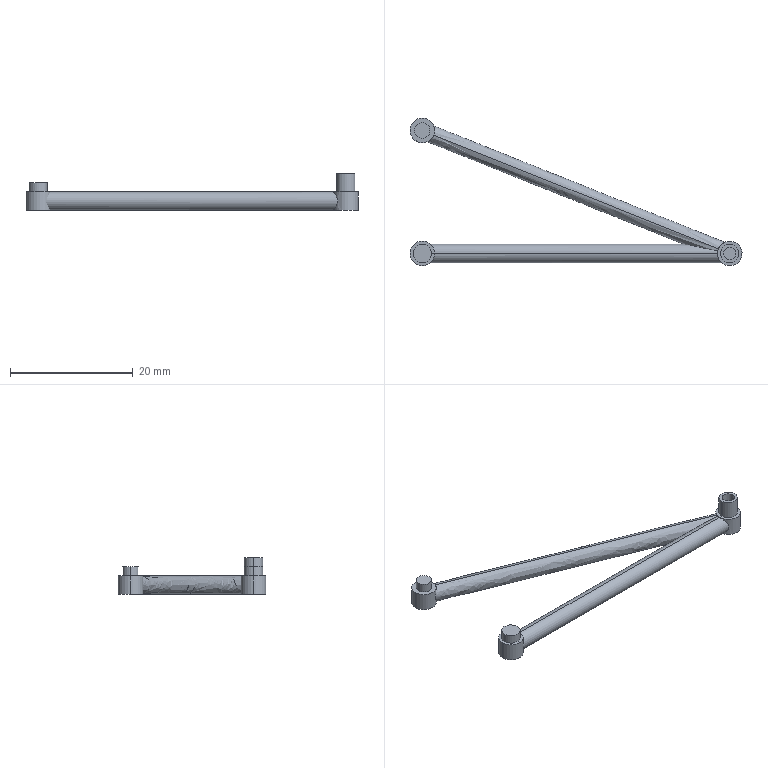Part | SolidWorks | features MirrorStock 1 | 3 solids | 36 faces | box 54 x 24 x 5.96 mm | volume 800.323 mm3 | cylinder 21 | plane 13 | spline 2 | commonest cylinder face diameters 4 x9 3 x6 0.5 x2 2 x2 2.5 x2
STEP:
#1=CARTESIAN_POINT('',(-2.,0.,-1.5));
#2=VERTEX_POINT('',#1);
#3=CARTESIAN_POINT('',(2.,0.,-1.5));
#4=VERTEX_POINT('',#3);
#5=CARTESIAN_POINT('',(0.,0.,-1.5));
#6=DIRECTION('',(0.,0.,1.));
#7=DIRECTION('',(1.,0.,0.));
#8=AXIS2_PLACEMENT_3D('',#5,#6,#7);
#9=CIRCLE('',#8,2.);
#10=EDGE_CURVE('',#2,#4,#9,.T.);
#11=ORIENTED_EDGE('',*,*,#10,.T.);
#12=CARTESIAN_POINT('',(2.,0.,1.5));
#13=VERTEX_POINT('',#12);
#14=CARTESIAN_POINT('',(2.,0.,-1.5));
#15=DIRECTION('',(0.,0.,1.));
#16=VECTOR('',#15,1000.);
#17=LINE('',#14,#16);
#18=EDGE_CURVE('',#4,#13,#17,.T.);
#19=ORIENTED_EDGE('',*,*,#18,.T.);
#20=CARTESIAN_POINT('',(-2.,0.,1.5));
#21=VERTEX_POINT('',#20);
#22=CARTESIAN_POINT('',(0.,0.,1.5));
#23=DIRECTION('',(0.,0.,1.));
#24=DIRECTION('',(1.,0.,0.));
#25=AXIS2_PLACEMENT_3D('',#22,#23,#24);
#26=CIRCLE('',#25,2.);
#27=EDGE_CURVE('',#21,#13,#26,.T.);
#28=ORIENTED_EDGE('',*,*,#27,.F.);
#29=CARTESIAN_POINT('',(-2.,0.,-1.5));
#30=DIRECTION('',(0.,0.,1.));
#31=VECTOR('',#30,1000.);
#32=LINE('',#29,#31);
#33=EDGE_CURVE('',#2,#21,#32,.T.);
#34=ORIENTED_EDGE('',*,*,#33,.F.);
#35=EDGE_LOOP('',(#11,#19,#28,#34));
#36=FACE_OUTER_BOUND('',#35,.T.);
#37=CARTESIAN_POINT('',(0.,0.,-1.5));
#38=DIRECTION('',(0.,0.,1.));
#39=DIRECTION('',(-1.,0.,0.));
#40=AXIS2_PLACEMENT_3D('',#37,#38,#39);
#41=CYLINDRICAL_SURFACE('',#40,2.);
#42=ADVANCED_FACE('',(#36),#41,.T.);
#43=ORIENTED_EDGE('',*,*,#18,.F.);
#44=CARTESIAN_POINT('',(0.,0.,-1.5));
#45=DIRECTION('',(0.,0.,1.));
#46=DIRECTION('',(1.,0.,0.));
#47=AXIS2_PLACEMENT_3D('',#44,#45,#46);
#48=CIRCLE('',#47,2.);
#49=EDGE_CURVE('',#4,#2,#48,.T.);
#50=ORIENTED_EDGE('',*,*,#49,.T.);
#51=ORIENTED_EDGE('',*,*,#33,.T.);
#52=CARTESIAN_POINT('',(0.,0.,1.5));
#53=DIRECTION('',(0.,0.,1.));
#54=DIRECTION('',(1.,0.,0.));
#55=AXIS2_PLACEMENT_3D('',#52,#53,#54);
#56=CIRCLE('',#55,2.);
#57=EDGE_CURVE('',#13,#21,#56,.T.);
#58=ORIENTED_EDGE('',*,*,#57,.F.);
#59=EDGE_LOOP('',(#43,#50,#51,#58));
#60=FACE_OUTER_BOUND('',#59,.T.);
#61=CARTESIAN_POINT('',(0.,0.,-1.5));
#62=DIRECTION('',(0.,0.,1.));
#63=DIRECTION('',(-1.,0.,0.));
#64=AXIS2_PLACEMENT_3D('',#61,#62,#63);
#65=CYLINDRICAL_SURFACE('',#64,2.);
#66=ADVANCED_FACE('',(#60),#65,.T.);
#67=ORIENTED_EDGE('',*,*,#10,.F.);
#68=ORIENTED_EDGE('',*,*,#49,.F.);
#69=EDGE_LOOP('',(#67,#68));
#70=FACE_OUTER_BOUND('',#69,.T.);
#71=CARTESIAN_POINT('',(0.,0.,-1.5));
#72=DIRECTION('',(0.,0.,-1.));
#73=DIRECTION('',(1.,0.,0.));
#74=AXIS2_PLACEMENT_3D('',#71,#72,#73);
#75=PLANE('',#74);
#76=ADVANCED_FACE('',(#70),#75,.T.);
#77=ORIENTED_EDGE('',*,*,#27,.T.);
#78=ORIENTED_EDGE('',*,*,#57,.T.);
#79=EDGE_LOOP('',(#77,#78));
#80=FACE_OUTER_BOUND('',#79,.T.);
#81=CARTESIAN_POINT('',(0.,0.,1.5));
#82=DIRECTION('',(0.,0.,-1.));
#83=DIRECTION('',(1.,0.,0.));
#84=AXIS2_PLACEMENT_3D('',#81,#82,#83);
#85=PLANE('',#84);
#86=ADVANCED_FACE('',(#80),#85,.F.);
#87=CLOSED_SHELL('',(#42,#66,#76,#86));
#88=MANIFOLD_SOLID_BREP('',#87);
#89=CARTESIAN_POINT('',(1.5,0.,3.));
#90=VERTEX_POINT('',#89);
#91=CARTESIAN_POINT('',(-1.5,0.,3.));
#92=VERTEX_POINT('',#91);
#93=CARTESIAN_POINT('',(0.,0.,3.));
#94=DIRECTION('',(0.,0.,-1.));
#95=DIRECTION('',(-1.,0.,0.));
#96=AXIS2_PLACEMENT_3D('',#93,#94,#95);
#97=CIRCLE('',#96,1.5);
#98=EDGE_CURVE('',#90,#92,#97,.T.);
#99=ORIENTED_EDGE('',*,*,#98,.T.);
#100=CARTESIAN_POINT('',(-1.5,0.,1.5));
#101=VERTEX_POINT('',#100);
#102=CARTESIAN_POINT('',(-1.5,0.,3.));
#103=DIRECTION('',(0.,0.,-1.));
#104=VECTOR('',#103,1000.);
#105=LINE('',#102,#104);
#106=EDGE_CURVE('',#92,#101,#105,.T.);
#107=ORIENTED_EDGE('',*,*,#106,.T.);
#108=CARTESIAN_POINT('',(1.5,0.,1.5));
#109=VERTEX_POINT('',#108);
#110=CARTESIAN_POINT('',(0.,0.,1.5));
#111=DIRECTION('',(0.,0.,-1.));
#112=DIRECTION('',(-1.,0.,0.));
#113=AXIS2_PLACEMENT_3D('',#110,#111,#112);
#114=CIRCLE('',#113,1.5);
#115=EDGE_CURVE('',#109,#101,#114,.T.);
#116=ORIENTED_EDGE('',*,*,#115,.F.);
#117=CARTESIAN_POINT('',(1.5,0.,3.));
#118=DIRECTION('',(0.,0.,-1.));
#119=VECTOR('',#118,1000.);
#120=LINE('',#117,#119);
#121=EDGE_CURVE('',#90,#109,#120,.T.);
#122=ORIENTED_EDGE('',*,*,#121,.F.);
#123=EDGE_LOOP('',(#99,#107,#116,#122));
#124=FACE_OUTER_BOUND('',#123,.T.);
#125=CARTESIAN_POINT('',(0.,0.,3.));
#126=DIRECTION('',(0.,0.,-1.));
#127=DIRECTION('',(1.,0.,0.));
#128=AXIS2_PLACEMENT_3D('',#125,#126,#127);
#129=CYLINDRICAL_SURFACE('',#128,1.5);
#130=ADVANCED_FACE('',(#124),#129,.T.);
#131=ORIENTED_EDGE('',*,*,#106,.F.);
#132=CARTESIAN_POINT('',(0.,0.,3.));
#133=DIRECTION('',(0.,0.,-1.));
#134=DIRECTION('',(-1.,0.,0.));
#135=AXIS2_PLACEMENT_3D('',#132,#133,#134);
#136=CIRCLE('',#135,1.5);
#137=EDGE_CURVE('',#92,#90,#136,.T.);
#138=ORIENTED_EDGE('',*,*,#137,.T.);
#139=ORIENTED_EDGE('',*,*,#121,.T.);
#140=CARTESIAN_POINT('',(0.,0.,1.5));
#141=DIRECTION('',(0.,0.,-1.));
#142=DIRECTION('',(-1.,0.,0.));
#143=AXIS2_PLACEMENT_3D('',#140,#141,#142);
#144=CIRCLE('',#143,1.5);
#145=EDGE_CURVE('',#101,#109,#144,.T.);
#146=ORIENTED_EDGE('',*,*,#145,.F.);
#147=EDGE_LOOP('',(#131,#138,#139,#146));
#148=FACE_OUTER_BOUND('',#147,.T.);
#149=CARTESIAN_POINT('',(0.,0.,3.));
#150=DIRECTION('',(0.,0.,-1.));
#151=DIRECTION('',(1.,0.,0.));
#152=AXIS2_PLACEMENT_3D('',#149,#150,#151);
#153=CYLINDRICAL_SURFACE('',#152,1.5);
#154=ADVANCED_FACE('',(#148),#153,.T.);
#155=ORIENTED_EDGE('',*,*,#98,.F.);
#156=ORIENTED_EDGE('',*,*,#137,.F.);
#157=EDGE_LOOP('',(#155,#156));
#158=FACE_OUTER_BOUND('',#157,.T.);
#159=CARTESIAN_POINT('',(0.,0.,3.));
#160=DIRECTION('',(0.,0.,1.));
#161=DIRECTION('',(-1.,0.,0.));
#162=AXIS2_PLACEMENT_3D('',#159,#160,#161);
#163=PLANE('',#162);
#164=ADVANCED_FACE('',(#158),#163,.T.);
#165=ORIENTED_EDGE('',*,*,#115,.T.);
#166=ORIENTED_EDGE('',*,*,#145,.T.);
#167=EDGE_LOOP('',(#165,#166));
#168=FACE_OUTER_BOUND('',#167,.T.);
#169=CARTESIAN_POINT('',(0.,0.,1.5));
#170=DIRECTION('',(0.,0.,1.));
#171=DIRECTION('',(-1.,0.,0.));
#172=AXIS2_PLACEMENT_3D('',#169,#170,#171);
#173=PLANE('',#172);
#174=ADVANCED_FACE('',(#168),#173,.F.);
#175=CLOSED_SHELL('',(#130,#154,#164,#174));
#176=MANIFOLD_SOLID_BREP('',#175);
#177=CARTESIAN_POINT('',(49.,0.,4.46));
#178=VERTEX_POINT('',#177);
#179=CARTESIAN_POINT('',(51.,0.,4.46));
#180=VERTEX_POINT('',#179);
#181=CARTESIAN_POINT('',(50.,0.,4.46));
#182=DIRECTION('',(0.,0.,-1.));
#183=DIRECTION('',(-1.,0.,0.));
#184=AXIS2_PLACEMENT_3D('',#181,#182,#183);
#185=CIRCLE('',#184,1.);
#186=EDGE_CURVE('',#178,#180,#185,.T.);
#187=ORIENTED_EDGE('',*,*,#186,.F.);
#188=CARTESIAN_POINT('',(49.,0.,1.5));
#189=VERTEX_POINT('',#188);
#190=CARTESIAN_POINT('',(49.,0.,4.46));
#191=DIRECTION('',(0.,0.,-1.));
#192=VECTOR('',#191,1000.);
#193=LINE('',#190,#192);
#194=EDGE_CURVE('',#178,#189,#193,.T.);
#195=ORIENTED_EDGE('',*,*,#194,.T.);
#196=CARTESIAN_POINT('',(51.,0.,1.5));
#197=VERTEX_POINT('',#196);
#198=CARTESIAN_POINT('',(50.,0.,1.5));
#199=DIRECTION('',(0.,0.,-1.));
#200=DIRECTION('',(-1.,0.,0.));
#201=AXIS2_PLACEMENT_3D('',#198,#199,#200);
#202=CIRCLE('',#201,1.);
#203=EDGE_CURVE('',#189,#197,#202,.T.);
#204=ORIENTED_EDGE('',*,*,#203,.T.);
#205=CARTESIAN_POINT('',(51.,0.,4.46));
#206=DIRECTION('',(0.,0.,-1.));
#207=VECTOR('',#206,1000.);
#208=LINE('',#205,#207);
#209=EDGE_CURVE('',#180,#197,#208,.T.);
#210=ORIENTED_EDGE('',*,*,#209,.F.);
#211=EDGE_LOOP('',(#187,#195,#204,#210));
#212=FACE_OUTER_BOUND('',#211,.T.);
#213=CARTESIAN_POINT('',(50.,0.,4.46));
#214=DIRECTION('',(0.,0.,-1.));
#215=DIRECTION('',(1.,0.,0.));
#216=AXIS2_PLACEMENT_3D('',#213,#214,#215);
#217=CYLINDRICAL_SURFACE('',#216,1.);
#218=ADVANCED_FACE('',(#212),#217,.F.);
#219=CARTESIAN_POINT('',(51.5,0.,4.46));
#220=VERTEX_POINT('',#219);
#221=CARTESIAN_POINT('',(48.5,0.,4.46));
#222=VERTEX_POINT('',#221);
#223=CARTESIAN_POINT('',(50.,0.,4.46));
#224=DIRECTION('',(0.,0.,-1.));
#225=DIRECTION('',(-1.,0.,0.));
#226=AXIS2_PLACEMENT_3D('',#223,#224,#225);
#227=CIRCLE('',#226,1.5);
#228=EDGE_CURVE('',#220,#222,#227,.T.);
#229=ORIENTED_EDGE('',*,*,#228,.T.);
#230=CARTESIAN_POINT('',(48.5,0.,1.5));
#231=VERTEX_POINT('',#230);
#232=CARTESIAN_POINT('',(48.5,0.,4.46));
#233=DIRECTION('',(0.,0.,-1.));
#234=VECTOR('',#233,1000.);
#235=LINE('',#232,#234);
#236=EDGE_CURVE('',#222,#231,#235,.T.);
#237=ORIENTED_EDGE('',*,*,#236,.T.);
#238=CARTESIAN_POINT('',(51.5,0.,1.5));
#239=VERTEX_POINT('',#238);
#240=CARTESIAN_POINT('',(50.,0.,1.5));
#241=DIRECTION('',(0.,0.,-1.));
#242=DIRECTION('',(1.,0.,0.));
#243=AXIS2_PLACEMENT_3D('',#240,#241,#242);
#244=CIRCLE('',#243,1.5);
#245=EDGE_CURVE('',#239,#231,#244,.T.);
#246=ORIENTED_EDGE('',*,*,#245,.F.);
#247=CARTESIAN_POINT('',(51.5,0.,4.46));
#248=DIRECTION('',(0.,0.,-1.));
#249=VECTOR('',#248,1000.);
#250=LINE('',#247,#249);
#251=EDGE_CURVE('',#220,#239,#250,.T.);
#252=ORIENTED_EDGE('',*,*,#251,.F.);
#253=EDGE_LOOP('',(#229,#237,#246,#252));
#254=FACE_OUTER_BOUND('',#253,.T.);
#255=CARTESIAN_POINT('',(50.,0.,4.46));
#256=DIRECTION('',(0.,0.,-1.));
#257=DIRECTION('',(1.,0.,0.));
#258=AXIS2_PLACEMENT_3D('',#255,#256,#257);
#259=CYLINDRICAL_SURFACE('',#258,1.5);
#260=ADVANCED_FACE('',(#254),#259,.T.);
#261=CARTESIAN_POINT('',(1.25,20.,3.));
#262=VERTEX_POINT('',#261);
#263=CARTESIAN_POINT('',(-1.25,20.,3.));
#264=VERTEX_POINT('',#263);
#265=CARTESIAN_POINT('',(0.,20.,3.));
#266=DIRECTION('',(0.,0.,-1.));
#267=DIRECTION('',(-1.,0.,0.));
#268=AXIS2_PLACEMENT_3D('',#265,#266,#267);
#269=CIRCLE('',#268,1.25);
#270=EDGE_CURVE('',#262,#264,#269,.T.);
#271=ORIENTED_EDGE('',*,*,#270,.T.);
#272=CARTESIAN_POINT('',(-1.25,20.,1.5));
#273=VERTEX_POINT('',#272);
#274=CARTESIAN_POINT('',(-1.25,20.,3.));
#275=DIRECTION('',(0.,0.,-1.));
#276=VECTOR('',#275,1000.);
#277=LINE('',#274,#276);
#278=EDGE_CURVE('',#264,#273,#277,.T.);
#279=ORIENTED_EDGE('',*,*,#278,.T.);
#280=CARTESIAN_POINT('',(1.25,20.,1.5));
#281=VERTEX_POINT('',#280);
#282=CARTESIAN_POINT('',(0.,20.,1.5));
#283=DIRECTION('',(0.,0.,-1.));
#284=DIRECTION('',(1.,0.,0.));
#285=AXIS2_PLACEMENT_3D('',#282,#283,#284);
#286=CIRCLE('',#285,1.25);
#287=EDGE_CURVE('',#281,#273,#286,.T.);
#288=ORIENTED_EDGE('',*,*,#287,.F.);
#289=CARTESIAN_POINT('',(1.25,20.,3.));
#290=DIRECTION('',(0.,0.,-1.));
#291=VECTOR('',#290,1000.);
#292=LINE('',#289,#291);
#293=EDGE_CURVE('',#262,#281,#292,.T.);
#294=ORIENTED_EDGE('',*,*,#293,.F.);
#295=EDGE_LOOP('',(#271,#279,#288,#294));
#296=FACE_OUTER_BOUND('',#295,.T.);
#297=CARTESIAN_POINT('',(0.,20.,3.));
#298=DIRECTION('',(0.,0.,-1.));
#299=DIRECTION('',(1.,0.,0.));
#300=AXIS2_PLACEMENT_3D('',#297,#298,#299);
#301=CYLINDRICAL_SURFACE('',#300,1.25);
#302=ADVANCED_FACE('',(#296),#301,.T.);
#303=CARTESIAN_POINT('',(49.75,0.,-1.5));
#304=VERTEX_POINT('',#303);
#305=CARTESIAN_POINT('',(50.25,0.,-1.5));
#306=VERTEX_POINT('',#305);
#307=CARTESIAN_POINT('',(50.,0.,-1.5));
#308=DIRECTION('',(0.,0.,-1.));
#309=DIRECTION('',(1.,0.,0.));
#310=AXIS2_PLACEMENT_3D('',#307,#308,#309);
#311=CIRCLE('',#310,0.25);
#312=EDGE_CURVE('',#304,#306,#311,.T.);
#313=ORIENTED_EDGE('',*,*,#312,.T.);
#314=CARTESIAN_POINT('',(50.25,0.,0.));
#315=VERTEX_POINT('',#314);
#316=CARTESIAN_POINT('',(50.25,0.,-4.));
#317=DIRECTION('',(0.,0.,1.));
#318=VECTOR('',#317,1000.);
#319=LINE('',#316,#318);
#320=EDGE_CURVE('',#306,#315,#319,.T.);
#321=ORIENTED_EDGE('',*,*,#320,.T.);
#322=CARTESIAN_POINT('',(49.75,0.,0.));
#323=VERTEX_POINT('',#322);
#324=CARTESIAN_POINT('',(50.,0.,0.));
#325=DIRECTION('',(0.,0.,1.));
#326=DIRECTION('',(1.,0.,0.));
#327=AXIS2_PLACEMENT_3D('',#324,#325,#326);
#328=CIRCLE('',#327,0.25);
#329=EDGE_CURVE('',#315,#323,#328,.T.);
#330=ORIENTED_EDGE('',*,*,#329,.T.);
#331=CARTESIAN_POINT('',(49.75,0.,-4.));
#332=DIRECTION('',(0.,0.,1.));
#333=VECTOR('',#332,1000.);
#334=LINE('',#331,#333);
#335=EDGE_CURVE('',#304,#323,#334,.T.);
#336=ORIENTED_EDGE('',*,*,#335,.F.);
#337=EDGE_LOOP('',(#313,#321,#330,#336));
#338=FACE_OUTER_BOUND('',#337,.T.);
#339=CARTESIAN_POINT('',(50.,0.,-4.));
#340=DIRECTION('',(0.,0.,1.));
#341=DIRECTION('',(-1.,0.,0.));
#342=AXIS2_PLACEMENT_3D('',#339,#340,#341);
#343=CYLINDRICAL_SURFACE('',#342,0.25);
#344=ADVANCED_FACE('',(#338),#343,.F.);
#345=CARTESIAN_POINT('',(1.857,19.257,-1.5));
#346=VERTEX_POINT('',#345);
#347=CARTESIAN_POINT('',(2.,20.,-1.5));
#348=VERTEX_POINT('',#347);
#349=CARTESIAN_POINT('',(0.,20.,-1.5));
#350=DIRECTION('',(0.,0.,1.));
#351=DIRECTION('',(1.,0.,0.));
#352=AXIS2_PLACEMENT_3D('',#349,#350,#351);
#353=CIRCLE('',#352,2.);
#354=EDGE_CURVE('',#346,#348,#353,.T.);
#355=ORIENTED_EDGE('',*,*,#354,.T.);
#356=CARTESIAN_POINT('',(2.,20.,-1.269));
#357=VERTEX_POINT('',#356);
#358=CARTESIAN_POINT('',(2.,20.,-1.5));
#359=DIRECTION('',(0.,0.,1.));
#360=VECTOR('',#359,1000.);
#361=LINE('',#358,#360);
#362=EDGE_CURVE('',#348,#357,#361,.T.);
#363=ORIENTED_EDGE('',*,*,#362,.T.);
#364=CARTESIAN_POINT('',(1.857,19.257,-1.5));
#365=CARTESIAN_POINT('',(1.907,19.381,-1.5));
#366=CARTESIAN_POINT('',(1.944,19.512,-1.479));
#367=CARTESIAN_POINT('',(1.99,19.763,-1.399));
#368=CARTESIAN_POINT('',(2.,19.887,-1.34));
#369=CARTESIAN_POINT('',(2.,20.,-1.269));
#370=B_SPLINE_CURVE_WITH_KNOTS('',3,(#364,#365,#366,#367,#368,#369),.UNSPECIFIED.,.F.,.F.,(4,2,4),(0.004731,0.005137,0.005543),.UNSPECIFIED.);
#371=EDGE_CURVE('',#346,#357,#370,.T.);
#372=ORIENTED_EDGE('',*,*,#371,.F.);
#373=EDGE_LOOP('',(#355,#363,#372));
#374=FACE_OUTER_BOUND('',#373,.T.);
#375=CARTESIAN_POINT('',(0.,20.,-1.5));
#376=DIRECTION('',(0.,0.,1.));
#377=DIRECTION('',(-1.,0.,0.));
#378=AXIS2_PLACEMENT_3D('',#375,#376,#377);
#379=CYLINDRICAL_SURFACE('',#378,2.);
#380=ADVANCED_FACE('',(#374),#379,.T.);
#381=CARTESIAN_POINT('',(2.,20.,1.269));
#382=VERTEX_POINT('',#381);
#383=CARTESIAN_POINT('',(1.857,19.257,1.5));
#384=VERTEX_POINT('',#383);
#385=CARTESIAN_POINT('',(2.,20.,1.269));
#386=CARTESIAN_POINT('',(2.,19.886,1.341));
#387=CARTESIAN_POINT('',(1.99,19.762,1.399));
#388=CARTESIAN_POINT('',(1.944,19.512,1.478));
#389=CARTESIAN_POINT('',(1.907,19.383,1.5));
#390=CARTESIAN_POINT('',(1.857,19.257,1.5));
#391=B_SPLINE_CURVE_WITH_KNOTS('',3,(#385,#386,#387,#388,#389,#390),.UNSPECIFIED.,.F.,.F.,(4,2,4),(0.008658,0.009063,0.009468),.UNSPECIFIED.);
#392=EDGE_CURVE('',#382,#384,#391,.T.);
#393=ORIENTED_EDGE('',*,*,#392,.F.);
#394=CARTESIAN_POINT('',(2.,20.,1.5));
#395=VERTEX_POINT('',#394);
#396=CARTESIAN_POINT('',(2.,20.,-1.5));
#397=DIRECTION('',(0.,0.,1.));
#398=VECTOR('',#397,1000.);
#399=LINE('',#396,#398);
#400=EDGE_CURVE('',#382,#395,#399,.T.);
#401=ORIENTED_EDGE('',*,*,#400,.T.);
#402=CARTESIAN_POINT('',(0.,20.,1.5));
#403=DIRECTION('',(0.,0.,1.));
#404=DIRECTION('',(1.,0.,0.));
#405=AXIS2_PLACEMENT_3D('',#402,#403,#404);
#406=CIRCLE('',#405,2.);
#407=EDGE_CURVE('',#384,#395,#406,.T.);
#408=ORIENTED_EDGE('',*,*,#407,.F.);
#409=EDGE_LOOP('',(#393,#401,#408));
#410=FACE_OUTER_BOUND('',#409,.T.);
#411=CARTESIAN_POINT('',(0.,20.,-1.5));
#412=DIRECTION('',(0.,0.,1.));
#413=DIRECTION('',(-1.,0.,0.));
#414=AXIS2_PLACEMENT_3D('',#411,#412,#413);
#415=CYLINDRICAL_SURFACE('',#414,2.);
#416=ADVANCED_FACE('',(#410),#415,.T.);
#417=ORIENTED_EDGE('',*,*,#362,.F.);
#418=CARTESIAN_POINT('',(-2.,20.,-1.5));
#419=VERTEX_POINT('',#418);
#420=CARTESIAN_POINT('',(0.,20.,-1.5));
#421=DIRECTION('',(0.,0.,1.));
#422=DIRECTION('',(1.,0.,0.));
#423=AXIS2_PLACEMENT_3D('',#420,#421,#422);
#424=CIRCLE('',#423,2.);
#425=EDGE_CURVE('',#348,#419,#424,.T.);
#426=ORIENTED_EDGE('',*,*,#425,.T.);
#427=CARTESIAN_POINT('',(-2.,20.,1.5));
#428=VERTEX_POINT('',#427);
#429=CARTESIAN_POINT('',(-2.,20.,-1.5));
#430=DIRECTION('',(0.,0.,1.));
#431=VECTOR('',#430,1000.);
#432=LINE('',#429,#431);
#433=EDGE_CURVE('',#419,#428,#432,.T.);
#434=ORIENTED_EDGE('',*,*,#433,.T.);
#435=CARTESIAN_POINT('',(0.,20.,1.5));
#436=DIRECTION('',(0.,0.,1.));
#437=DIRECTION('',(1.,0.,0.));
#438=AXIS2_PLACEMENT_3D('',#435,#436,#437);
#439=CIRCLE('',#438,2.);
#440=EDGE_CURVE('',#395,#428,#439,.T.);
#441=ORIENTED_EDGE('',*,*,#440,.F.);
#442=ORIENTED_EDGE('',*,*,#400,.F.);
#443=CARTESIAN_POINT('',(2.,20.,-1.269));
#444=CARTESIAN_POINT('',(2.,20.218,-1.132));
#445=CARTESIAN_POINT('',(1.963,20.406,-0.9449));
#446=CARTESIAN_POINT('',(1.906,20.609,-0.6191));
#447=CARTESIAN_POINT('',(1.887,20.664,-0.5023));
#448=CARTESIAN_POINT('',(1.858,20.74,-0.2559));
#449=CARTESIAN_POINT('',(1.85,20.76,-0.1291));
#450=CARTESIAN_POINT('',(1.85,20.76,0.129));
#451=CARTESIAN_POINT('',(1.859,20.739,0.2594));
#452=CARTESIAN_POINT('',(1.887,20.664,0.5037));
#453=CARTESIAN_POINT('',(1.906,20.609,0.6202));
#454=CARTESIAN_POINT('',(1.964,20.405,0.9457));
#455=CARTESIAN_POINT('',(2.,20.219,1.131));
#456=CARTESIAN_POINT('',(2.,20.,1.269));
#457=B_SPLINE_CURVE_WITH_KNOTS('',3,(#443,#444,#445,#446,#447,#448,#449,#450,#451,#452,#453,#454,#455,#456),.UNSPECIFIED.,.F.,.F.,(4,2,2,2,2,2,4),(0.005543,0.006322,0.006711,0.0071,0.00749,0.007879,0.008658),.UNSPECIFIED.);
#458=EDGE_CURVE('',#357,#382,#457,.T.);
#459=ORIENTED_EDGE('',*,*,#458,.F.);
#460=EDGE_LOOP('',(#417,#426,#434,#441,#442,#459));
#461=FACE_OUTER_BOUND('',#460,.T.);
#462=CARTESIAN_POINT('',(0.,20.,-1.5));
#463=DIRECTION('',(0.,0.,1.));
#464=DIRECTION('',(-1.,0.,0.));
#465=AXIS2_PLACEMENT_3D('',#462,#463,#464);
#466=CYLINDRICAL_SURFACE('',#465,2.);
#467=ADVANCED_FACE('',(#461),#466,.T.);
#468=CARTESIAN_POINT('',(48.,0.,-1.5));
#469=VERTEX_POINT('',#468);
#470=CARTESIAN_POINT('',(48.,0.,1.5));
#471=VERTEX_POINT('',#470);
#472=CARTESIAN_POINT('',(48.,0.,-1.5));
#473=CARTESIAN_POINT('',(48.,-0.104,-1.5));
#474=CARTESIAN_POINT('',(48.008,-0.2056,-1.489));
#475=CARTESIAN_POINT('',(48.039,-0.4042,-1.448));
#476=CARTESIAN_POINT('',(48.062,-0.5017,-1.417));
#477=CARTESIAN_POINT('',(48.146,-0.7738,-1.3));
#478=CARTESIAN_POINT('',(48.225,-0.934,-1.189));
#479=CARTESIAN_POINT('',(48.391,-1.199,-0.9211));
#480=CARTESIAN_POINT('',(48.48,-1.304,-0.7655));
#481=CARTESIAN_POINT('',(48.588,-1.418,-0.4991));
#482=CARTESIAN_POINT('',(48.62,-1.448,-0.4042));
#483=CARTESIAN_POINT('',(48.664,-1.489,-0.2077));
#484=CARTESIAN_POINT('',(48.677,-1.5,-0.1035));
#485=CARTESIAN_POINT('',(48.677,-1.5,0.1012));
#486=CARTESIAN_POINT('',(48.665,-1.489,0.2047));
#487=CARTESIAN_POINT('',(48.621,-1.449,0.4023));
#488=CARTESIAN_POINT('',(48.589,-1.419,0.497));
#489=CARTESIAN_POINT('',(48.517,-1.343,0.6752));
#490=CARTESIAN_POINT('',(48.477,-1.298,0.758));
#491=CARTESIAN_POINT('',(48.394,-1.193,0.9137));
#492=CARTESIAN_POINT('',(48.35,-1.133,0.9872));
#493=CARTESIAN_POINT('',(48.267,-1.001,1.121));
#494=CARTESIAN_POINT('',(48.227,-0.929,1.182));
#495=CARTESIAN_POINT('',(48.153,-0.7712,1.29));
#496=CARTESIAN_POINT('',(48.118,-0.6846,1.338));
#497=CARTESIAN_POINT('',(48.034,-0.4127,1.456));
#498=CARTESIAN_POINT('',(48.,-0.2082,1.5));
#499=CARTESIAN_POINT('',(48.,0.,1.5));
#500=B_SPLINE_CURVE_WITH_KNOTS('',3,(#472,#473,#474,#475,#476,#477,#478,#479,#480,#481,#482,#483,#484,#485,#486,#487,#488,#489,#490,#491,#492,#493,#494,#495,#496,#497,#498,#499),.UNSPECIFIED.,.F.,.F.,(4,2,2,2,2,2,2,2,2,2,2,2,2,4),(0.,0.0003069,0.0006138,0.001228,0.001841,0.002148,0.002455,0.002762,0.003069,0.003376,0.003683,0.00399,0.004297,0.004911),.UNSPECIFIED.);
#501=EDGE_CURVE('',#469,#471,#500,.T.);
#502=ORIENTED_EDGE('',*,*,#501,.T.);
#503=CARTESIAN_POINT('',(0.,0.,1.5));
#504=VERTEX_POINT('',#503);
#505=CARTESIAN_POINT('',(50.,0.,1.5));
#506=DIRECTION('',(-1.,0.,0.));
#507=VECTOR('',#506,1000.);
#508=LINE('',#505,#507);
#509=EDGE_CURVE('',#471,#504,#508,.T.);
#510=ORIENTED_EDGE('',*,*,#509,.T.);
#511=CARTESIAN_POINT('',(0.,0.,-1.5));
#512=VERTEX_POINT('',#511);
#513=CARTESIAN_POINT('',(0.,0.,0.));
#514=DIRECTION('',(-1.,0.,0.));
#515=DIRECTION('',(0.,0.,1.));
#516=AXIS2_PLACEMENT_3D('',#513,#514,#515);
#517=CIRCLE('',#516,1.5);
#518=EDGE_CURVE('',#512,#504,#517,.T.);
#519=ORIENTED_EDGE('',*,*,#518,.F.);
#520=CARTESIAN_POINT('',(50.,0.,-1.5));
#521=DIRECTION('',(-1.,0.,0.));
#522=VECTOR('',#521,1000.);
#523=LINE('',#520,#522);
#524=EDGE_CURVE('',#469,#512,#523,.T.);
#525=ORIENTED_EDGE('',*,*,#524,.F.);
#526=EDGE_LOOP('',(#502,#510,#519,#525));
#527=FACE_OUTER_BOUND('',#526,.T.);
#528=CARTESIAN_POINT('',(50.,0.,0.));
#529=DIRECTION('',(-1.,0.,0.));
#530=DIRECTION('',(0.,0.,-1.));
#531=AXIS2_PLACEMENT_3D('',#528,#529,#530);
#532=CYLINDRICAL_SURFACE('',#531,1.5);
#533=ADVANCED_FACE('',(#527),#532,.T.);
#534=CARTESIAN_POINT('',(48.143,0.7428,1.5));
#535=VERTEX_POINT('',#534);
#536=CARTESIAN_POINT('',(48.143,0.7428,-1.5));
#537=VERTEX_POINT('',#536);
#538=CARTESIAN_POINT('',(48.143,0.7428,1.5));
#539=CARTESIAN_POINT('',(48.18,0.8348,1.5));
#540=CARTESIAN_POINT('',(48.223,0.9218,1.489));
#541=CARTESIAN_POINT('',(48.318,1.087,1.445));
#542=CARTESIAN_POINT('',(48.372,1.165,1.413));
#543=CARTESIAN_POINT('',(48.536,1.375,1.291));
#544=CARTESIAN_POINT('',(48.656,1.487,1.176));
#545=CARTESIAN_POINT('',(48.878,1.662,0.9026));
#546=CARTESIAN_POINT('',(48.982,1.724,0.7432));
#547=CARTESIAN_POINT('',(49.137,1.806,0.3895));
#548=CARTESIAN_POINT('',(49.185,1.826,0.193));
#549=CARTESIAN_POINT('',(49.184,1.826,-0.09937));
#550=CARTESIAN_POINT('',(49.173,1.821,-0.1976));
#551=CARTESIAN_POINT('',(49.129,1.801,-0.3879));
#552=CARTESIAN_POINT('',(49.098,1.785,-0.4791));
#553=CARTESIAN_POINT('',(48.982,1.724,-0.7434));
#554=CARTESIAN_POINT('',(48.877,1.661,-0.9035));
#555=CARTESIAN_POINT('',(48.656,1.488,-1.176));
#556=CARTESIAN_POINT('',(48.537,1.375,-1.291));
#557=CARTESIAN_POINT('',(48.318,1.096,-1.453));
#558=CARTESIAN_POINT('',(48.215,0.9239,-1.5));
#559=CARTESIAN_POINT('',(48.143,0.7428,-1.5));
#560=B_SPLINE_CURVE_WITH_KNOTS('',3,(#538,#539,#540,#541,#542,#543,#544,#545,#546,#547,#548,#549,#550,#551,#552,#553,#554,#555,#556,#557,#558,#559),.UNSPECIFIED.,.F.,.F.,(4,2,2,2,2,2,2,2,2,2,4),(0.,0.0002925,0.0005849,0.00117,0.001755,0.00234,0.002632,0.002925,0.003509,0.004094,0.004679),.UNSPECIFIED.);
#561=EDGE_CURVE('',#535,#537,#560,.T.);
#562=ORIENTED_EDGE('',*,*,#561,.T.);
#563=CARTESIAN_POINT('',(50.138,-0.0551,-1.5));
#564=DIRECTION('',(-0.9285,0.3714,0.));
#565=VECTOR('',#564,1000.);
#566=LINE('',#563,#565);
#567=EDGE_CURVE('',#537,#346,#566,.T.);
#568=ORIENTED_EDGE('',*,*,#567,.T.);
#569=ORIENTED_EDGE('',*,*,#371,.T.);
#570=ORIENTED_EDGE('',*,*,#458,.T.);
#571=ORIENTED_EDGE('',*,*,#392,.T.);
#572=CARTESIAN_POINT('',(50.138,-0.0551,1.5));
#573=DIRECTION('',(-0.9285,0.3714,0.));
#574=VECTOR('',#573,1000.);
#575=LINE('',#572,#574);
#576=EDGE_CURVE('',#535,#384,#575,.T.);
#577=ORIENTED_EDGE('',*,*,#576,.F.);
#578=EDGE_LOOP('',(#562,#568,#569,#570,#571,#577));
#579=FACE_OUTER_BOUND('',#578,.T.);
#580=CARTESIAN_POINT('',(49.475,0.2101,-1.5));
#581=CARTESIAN_POINT('',(1.564,19.374,-1.5));
#582=CARTESIAN_POINT('',(49.475,3.21,-1.5));
#583=CARTESIAN_POINT('',(1.564,22.374,-1.5));
#584=CARTESIAN_POINT('',(49.475,3.21,1.5));
#585=CARTESIAN_POINT('',(1.564,22.374,1.5));
#586=CARTESIAN_POINT('',(49.475,0.2101,1.5));
#587=CARTESIAN_POINT('',(1.564,19.374,1.5));
#588=(BOUNDED_SURFACE()B_SPLINE_SURFACE(3,1,((#580,#581),(#582,#583),(#584,#585),(#586,#587)),.UNSPECIFIED.,.F.,.F.,.F.)B_SPLINE_SURFACE_WITH_KNOTS((4,4),(2,2),(0.,1.),(0.,1.),.UNSPECIFIED.)GEOMETRIC_REPRESENTATION_ITEM()RATIONAL_B_SPLINE_SURFACE(((1.,1.),(0.3333,0.3333),(0.3333,0.3333),(1.,1.)))REPRESENTATION_ITEM('')SURFACE());
#589=ADVANCED_FACE('',(#579),#588,.T.);
#590=ORIENTED_EDGE('',*,*,#567,.F.);
#591=CARTESIAN_POINT('',(48.039,0.3922,-1.448));
#592=VERTEX_POINT('',#591);
#593=CARTESIAN_POINT('',(48.143,0.7428,-1.5));
#594=CARTESIAN_POINT('',(48.12,0.6856,-1.5));
#595=CARTESIAN_POINT('',(48.1,0.6275,-1.496));
#596=CARTESIAN_POINT('',(48.065,0.509,-1.478));
#597=CARTESIAN_POINT('',(48.05,0.4503,-1.465));
#598=CARTESIAN_POINT('',(48.039,0.3922,-1.448));
#599=B_SPLINE_CURVE_WITH_KNOTS('',3,(#593,#594,#595,#596,#597,#598),.UNSPECIFIED.,.F.,.F.,(4,2,4),(0.004679,0.004864,0.005048),.UNSPECIFIED.);
#600=EDGE_CURVE('',#537,#592,#599,.T.);
#601=ORIENTED_EDGE('',*,*,#600,.T.);
#602=CARTESIAN_POINT('',(48.039,0.3922,1.448));
#603=VERTEX_POINT('',#602);
#604=CARTESIAN_POINT('',(48.039,0.3922,-1.448));
#605=CARTESIAN_POINT('',(47.547,0.4906,-1.421));
#606=CARTESIAN_POINT('',(47.056,0.5889,-1.384));
#607=CARTESIAN_POINT('',(46.076,0.7849,-1.283));
#608=CARTESIAN_POINT('',(45.587,0.8826,-1.22));
#609=CARTESIAN_POINT('',(44.615,1.077,-1.052));
#610=CARTESIAN_POINT('',(44.132,1.174,-0.9505));
#611=CARTESIAN_POINT('',(43.426,1.315,-0.7275));
#612=CARTESIAN_POINT('',(43.193,1.361,-0.6418));
#613=CARTESIAN_POINT('',(42.868,1.426,-0.4679));
#614=CARTESIAN_POINT('',(42.761,1.448,-0.4019));
#615=CARTESIAN_POINT('',(42.623,1.475,-0.2745));
#616=CARTESIAN_POINT('',(42.581,1.484,-0.2267));
#617=CARTESIAN_POINT('',(42.518,1.496,-0.1182));
#618=CARTESIAN_POINT('',(42.498,1.5,-0.05508));
#619=CARTESIAN_POINT('',(42.502,1.5,0.0716));
#620=CARTESIAN_POINT('',(42.525,1.495,0.1328));
#621=CARTESIAN_POINT('',(42.591,1.482,0.2396));
#622=CARTESIAN_POINT('',(42.634,1.473,0.2858));
#623=CARTESIAN_POINT('',(42.774,1.445,0.4104));
#624=CARTESIAN_POINT('',(42.88,1.424,0.4754));
#625=CARTESIAN_POINT('',(43.206,1.359,0.647));
#626=CARTESIAN_POINT('',(43.439,1.312,0.7319));
#627=CARTESIAN_POINT('',(44.143,1.171,0.953));
#628=CARTESIAN_POINT('',(44.625,1.075,1.054));
#629=CARTESIAN_POINT('',(45.593,0.8813,1.22));
#630=CARTESIAN_POINT('',(46.081,0.7838,1.284));
#631=CARTESIAN_POINT('',(47.058,0.5883,1.384));
#632=CARTESIAN_POINT('',(47.548,0.4903,1.421));
#633=CARTESIAN_POINT('',(48.039,0.3922,1.448));
#634=B_SPLINE_CURVE_WITH_KNOTS('',3,(#604,#605,#606,#607,#608,#609,#610,#611,#612,#613,#614,#615,#616,#617,#618,#619,#620,#621,#622,#623,#624,#625,#626,#627,#628,#629,#630,#631,#632,#633),.UNSPECIFIED.,.F.,.F.,(4,2,2,2,2,2,2,2,2,2,2,2,2,2,4),(0.001987,0.003494,0.005001,0.006508,0.007261,0.007638,0.007826,0.008015,0.008203,0.008391,0.008768,0.009522,0.01103,0.01254,0.01404),.UNSPECIFIED.);
#635=EDGE_CURVE('',#592,#603,#634,.T.);
#636=ORIENTED_EDGE('',*,*,#635,.T.);
#637=CARTESIAN_POINT('',(48.039,0.3922,1.448));
#638=CARTESIAN_POINT('',(48.05,0.4502,1.465));
#639=CARTESIAN_POINT('',(48.065,0.5093,1.478));
#640=CARTESIAN_POINT('',(48.1,0.6268,1.496));
#641=CARTESIAN_POINT('',(48.12,0.6851,1.5));
#642=CARTESIAN_POINT('',(48.143,0.7428,1.5));
#643=B_SPLINE_CURVE_WITH_KNOTS('',3,(#637,#638,#639,#640,#641,#642),.UNSPECIFIED.,.F.,.F.,(4,2,4),(0.008993,0.009176,0.009359),.UNSPECIFIED.);
#644=EDGE_CURVE('',#603,#535,#643,.T.);
#645=ORIENTED_EDGE('',*,*,#644,.T.);
#646=ORIENTED_EDGE('',*,*,#576,.T.);
#647=CARTESIAN_POINT('',(1.857,19.257,1.5));
#648=CARTESIAN_POINT('',(1.82,19.165,1.5));
#649=CARTESIAN_POINT('',(1.777,19.076,1.488));
#650=CARTESIAN_POINT('',(1.681,18.911,1.445));
#651=CARTESIAN_POINT('',(1.628,18.835,1.413));
#652=CARTESIAN_POINT('',(1.462,18.623,1.29));
#653=CARTESIAN_POINT('',(1.343,18.512,1.176));
#654=CARTESIAN_POINT('',(1.121,18.337,0.9009));
#655=CARTESIAN_POINT('',(1.018,18.276,0.7433));
#656=CARTESIAN_POINT('',(0.8634,18.194,0.3903));
#657=CARTESIAN_POINT('',(0.8154,18.174,0.1942));
#658=CARTESIAN_POINT('',(0.8155,18.174,-0.09799));
#659=CARTESIAN_POINT('',(0.8272,18.179,-0.1969));
#660=CARTESIAN_POINT('',(0.8705,18.199,-0.3865));
#661=CARTESIAN_POINT('',(0.9018,18.214,-0.4782));
#662=CARTESIAN_POINT('',(1.018,18.276,-0.7431));
#663=CARTESIAN_POINT('',(1.122,18.338,-0.9023));
#664=CARTESIAN_POINT('',(1.344,18.512,-1.176));
#665=CARTESIAN_POINT('',(1.463,18.625,-1.291));
#666=CARTESIAN_POINT('',(1.629,18.837,-1.414));
#667=CARTESIAN_POINT('',(1.682,18.913,-1.445));
#668=CARTESIAN_POINT('',(1.777,19.078,-1.489));
#669=CARTESIAN_POINT('',(1.821,19.167,-1.5));
#670=CARTESIAN_POINT('',(1.857,19.257,-1.5));
#671=B_SPLINE_CURVE_WITH_KNOTS('',3,(#647,#648,#649,#650,#651,#652,#653,#654,#655,#656,#657,#658,#659,#660,#661,#662,#663,#664,#665,#666,#667,#668,#669,#670),.UNSPECIFIED.,.F.,.F.,(4,2,2,2,2,2,2,2,2,2,2,4),(0.,0.0002957,0.0005914,0.001183,0.001774,0.002366,0.002661,0.002957,0.003548,0.00414,0.004435,0.004731),.UNSPECIFIED.);
#672=EDGE_CURVE('',#384,#346,#671,.T.);
#673=ORIENTED_EDGE('',*,*,#672,.T.);
#674=EDGE_LOOP('',(#590,#601,#636,#645,#646,#673));
#675=FACE_OUTER_BOUND('',#674,.T.);
#676=CARTESIAN_POINT('',(48.427,0.6292,1.5));
#677=CARTESIAN_POINT('',(0.5254,19.79,1.5));
#678=CARTESIAN_POINT('',(48.427,-2.371,1.5));
#679=CARTESIAN_POINT('',(0.5254,16.79,1.5));
#680=CARTESIAN_POINT('',(48.427,-2.371,-1.5));
#681=CARTESIAN_POINT('',(0.5254,16.79,-1.5));
#682=CARTESIAN_POINT('',(48.427,0.6292,-1.5));
#683=CARTESIAN_POINT('',(0.5254,19.79,-1.5));
#684=(BOUNDED_SURFACE()B_SPLINE_SURFACE(3,1,((#676,#677),(#678,#679),(#680,#681),(#682,#683)),.UNSPECIFIED.,.F.,.F.,.F.)B_SPLINE_SURFACE_WITH_KNOTS((4,4),(2,2),(0.,1.),(0.,1.),.UNSPECIFIED.)GEOMETRIC_REPRESENTATION_ITEM()RATIONAL_B_SPLINE_SURFACE(((1.,1.),(0.3333,0.3333),(0.3333,0.3333),(1.,1.)))REPRESENTATION_ITEM('')SURFACE());
#685=ADVANCED_FACE('',(#675),#684,.T.);
#686=ORIENTED_EDGE('',*,*,#509,.F.);
#687=CARTESIAN_POINT('',(48.,0.,1.5));
#688=CARTESIAN_POINT('',(48.,0.1347,1.5));
#689=CARTESIAN_POINT('',(48.013,0.2653,1.482));
#690=CARTESIAN_POINT('',(48.039,0.3922,1.448));
#691=B_SPLINE_CURVE_WITH_KNOTS('',3,(#687,#688,#689,#690),.UNSPECIFIED.,.F.,.F.,(4,4),(0.,0.0003975),.UNSPECIFIED.);
#692=EDGE_CURVE('',#471,#603,#691,.T.);
#693=ORIENTED_EDGE('',*,*,#692,.T.);
#694=ORIENTED_EDGE('',*,*,#635,.F.);
#695=CARTESIAN_POINT('',(48.039,0.3922,-1.448));
#696=CARTESIAN_POINT('',(48.014,0.2662,-1.482));
#697=CARTESIAN_POINT('',(48.,0.1339,-1.5));
#698=CARTESIAN_POINT('',(48.,0.,-1.5));
#699=B_SPLINE_CURVE_WITH_KNOTS('',3,(#695,#696,#697,#698),.UNSPECIFIED.,.F.,.F.,(4,4),(0.004516,0.004911),.UNSPECIFIED.);
#700=EDGE_CURVE('',#592,#469,#699,.T.);
#701=ORIENTED_EDGE('',*,*,#700,.T.);
#702=ORIENTED_EDGE('',*,*,#524,.T.);
#703=CARTESIAN_POINT('',(0.,0.,0.));
#704=DIRECTION('',(-1.,0.,0.));
#705=DIRECTION('',(0.,0.,1.));
#706=AXIS2_PLACEMENT_3D('',#703,#704,#705);
#707=CIRCLE('',#706,1.5);
#708=EDGE_CURVE('',#504,#512,#707,.T.);
#709=ORIENTED_EDGE('',*,*,#708,.F.);
#710=EDGE_LOOP('',(#686,#693,#694,#701,#702,#709));
#711=FACE_OUTER_BOUND('',#710,.T.);
#712=CARTESIAN_POINT('',(50.,0.,0.));
#713=DIRECTION('',(-1.,0.,0.));
#714=DIRECTION('',(0.,0.,-1.));
#715=AXIS2_PLACEMENT_3D('',#712,#713,#714);
#716=CYLINDRICAL_SURFACE('',#715,1.5);
#717=ADVANCED_FACE('',(#711),#716,.T.);
#718=ORIENTED_EDGE('',*,*,#518,.T.);
#719=ORIENTED_EDGE('',*,*,#708,.T.);
#720=EDGE_LOOP('',(#718,#719));
#721=FACE_OUTER_BOUND('',#720,.T.);
#722=CARTESIAN_POINT('',(0.,0.,0.));
#723=DIRECTION('',(1.,0.,0.));
#724=DIRECTION('',(0.,0.,1.));
#725=AXIS2_PLACEMENT_3D('',#722,#723,#724);
#726=PLANE('',#725);
#727=ADVANCED_FACE('',(#721),#726,.F.);
#728=ORIENTED_EDGE('',*,*,#433,.F.);
#729=CARTESIAN_POINT('',(0.,20.,-1.5));
#730=DIRECTION('',(0.,0.,1.));
#731=DIRECTION('',(1.,0.,0.));
#732=AXIS2_PLACEMENT_3D('',#729,#730,#731);
#733=CIRCLE('',#732,2.);
#734=EDGE_CURVE('',#419,#346,#733,.T.);
#735=ORIENTED_EDGE('',*,*,#734,.T.);
#736=ORIENTED_EDGE('',*,*,#672,.F.);
#737=CARTESIAN_POINT('',(0.,20.,1.5));
#738=DIRECTION('',(0.,0.,1.));
#739=DIRECTION('',(1.,0.,0.));
#740=AXIS2_PLACEMENT_3D('',#737,#738,#739);
#741=CIRCLE('',#740,2.);
#742=EDGE_CURVE('',#428,#384,#741,.T.);
#743=ORIENTED_EDGE('',*,*,#742,.F.);
#744=EDGE_LOOP('',(#728,#735,#736,#743));
#745=FACE_OUTER_BOUND('',#744,.T.);
#746=CARTESIAN_POINT('',(0.,20.,-1.5));
#747=DIRECTION('',(0.,0.,1.));
#748=DIRECTION('',(-1.,0.,0.));
#749=AXIS2_PLACEMENT_3D('',#746,#747,#748);
#750=CYLINDRICAL_SURFACE('',#749,2.);
#751=ADVANCED_FACE('',(#745),#750,.T.);
#752=ORIENTED_EDGE('',*,*,#354,.F.);
#753=ORIENTED_EDGE('',*,*,#734,.F.);
#754=ORIENTED_EDGE('',*,*,#425,.F.);
#755=EDGE_LOOP('',(#752,#753,#754));
#756=FACE_OUTER_BOUND('',#755,.T.);
#757=CARTESIAN_POINT('',(0.,20.,-1.5));
#758=DIRECTION('',(0.,0.,-1.));
#759=DIRECTION('',(1.,0.,0.));
#760=AXIS2_PLACEMENT_3D('',#757,#758,#759);
#761=PLANE('',#760);
#762=ADVANCED_FACE('',(#756),#761,.T.);
#763=ORIENTED_EDGE('',*,*,#287,.T.);
#764=CARTESIAN_POINT('',(0.,20.,1.5));
#765=DIRECTION('',(0.,0.,-1.));
#766=DIRECTION('',(1.,0.,0.));
#767=AXIS2_PLACEMENT_3D('',#764,#765,#766);
#768=CIRCLE('',#767,1.25);
#769=EDGE_CURVE('',#273,#281,#768,.T.);
#770=ORIENTED_EDGE('',*,*,#769,.T.);
#771=EDGE_LOOP('',(#763,#770));
#772=FACE_BOUND('',#771,.T.);
#773=ORIENTED_EDGE('',*,*,#407,.T.);
#774=ORIENTED_EDGE('',*,*,#440,.T.);
#775=ORIENTED_EDGE('',*,*,#742,.T.);
#776=EDGE_LOOP('',(#773,#774,#775));
#777=FACE_OUTER_BOUND('',#776,.T.);
#778=CARTESIAN_POINT('',(0.,20.,1.5));
#779=DIRECTION('',(0.,0.,-1.));
#780=DIRECTION('',(1.,0.,0.));
#781=AXIS2_PLACEMENT_3D('',#778,#779,#780);
#782=PLANE('',#781);
#783=ADVANCED_FACE('',(#772,#777),#782,.F.);
#784=ORIENTED_EDGE('',*,*,#692,.F.);
#785=CARTESIAN_POINT('',(50.,0.,1.5));
#786=DIRECTION('',(0.,0.,1.));
#787=DIRECTION('',(1.,0.,0.));
#788=AXIS2_PLACEMENT_3D('',#785,#786,#787);
#789=CIRCLE('',#788,2.);
#790=EDGE_CURVE('',#535,#471,#789,.T.);
#791=ORIENTED_EDGE('',*,*,#790,.F.);
#792=ORIENTED_EDGE('',*,*,#644,.F.);
#793=EDGE_LOOP('',(#784,#791,#792));
#794=FACE_OUTER_BOUND('',#793,.T.);
#795=CARTESIAN_POINT('',(50.,0.,-1.5));
#796=DIRECTION('',(0.,0.,1.));
#797=DIRECTION('',(-1.,0.,0.));
#798=AXIS2_PLACEMENT_3D('',#795,#796,#797);
#799=CYLINDRICAL_SURFACE('',#798,2.);
#800=ADVANCED_FACE('',(#794),#799,.T.);
#801=CARTESIAN_POINT('',(50.,0.,1.5));
#802=DIRECTION('',(0.,0.,1.));
#803=DIRECTION('',(1.,0.,0.));
#804=AXIS2_PLACEMENT_3D('',#801,#802,#803);
#805=CIRCLE('',#804,2.);
#806=EDGE_CURVE('',#471,#535,#805,.T.);
#807=ORIENTED_EDGE('',*,*,#806,.F.);
#808=ORIENTED_EDGE('',*,*,#501,.F.);
#809=CARTESIAN_POINT('',(50.,0.,-1.5));
#810=DIRECTION('',(0.,0.,1.));
#811=DIRECTION('',(1.,0.,0.));
#812=AXIS2_PLACEMENT_3D('',#809,#810,#811);
#813=CIRCLE('',#812,2.);
#814=EDGE_CURVE('',#469,#537,#813,.T.);
#815=ORIENTED_EDGE('',*,*,#814,.T.);
#816=ORIENTED_EDGE('',*,*,#561,.F.);
#817=EDGE_LOOP('',(#807,#808,#815,#816));
#818=FACE_OUTER_BOUND('',#817,.T.);
#819=CARTESIAN_POINT('',(50.,0.,-1.5));
#820=DIRECTION('',(0.,0.,1.));
#821=DIRECTION('',(-1.,0.,0.));
#822=AXIS2_PLACEMENT_3D('',#819,#820,#821);
#823=CYLINDRICAL_SURFACE('',#822,2.);
#824=ADVANCED_FACE('',(#818),#823,.T.);
#825=CARTESIAN_POINT('',(50.,0.,-1.5));
#826=DIRECTION('',(0.,0.,1.));
#827=DIRECTION('',(1.,0.,0.));
#828=AXIS2_PLACEMENT_3D('',#825,#826,#827);
#829=CIRCLE('',#828,2.);
#830=EDGE_CURVE('',#537,#469,#829,.T.);
#831=ORIENTED_EDGE('',*,*,#830,.T.);
#832=ORIENTED_EDGE('',*,*,#700,.F.);
#833=ORIENTED_EDGE('',*,*,#600,.F.);
#834=EDGE_LOOP('',(#831,#832,#833));
#835=FACE_OUTER_BOUND('',#834,.T.);
#836=CARTESIAN_POINT('',(50.,0.,-1.5));
#837=DIRECTION('',(0.,0.,1.));
#838=DIRECTION('',(-1.,0.,0.));
#839=AXIS2_PLACEMENT_3D('',#836,#837,#838);
#840=CYLINDRICAL_SURFACE('',#839,2.);
#841=ADVANCED_FACE('',(#835),#840,.T.);
#842=ORIENTED_EDGE('',*,*,#312,.F.);
#843=CARTESIAN_POINT('',(50.,0.,-1.5));
#844=DIRECTION('',(0.,0.,-1.));
#845=DIRECTION('',(1.,0.,0.));
#846=AXIS2_PLACEMENT_3D('',#843,#844,#845);
#847=CIRCLE('',#846,0.25);
#848=EDGE_CURVE('',#306,#304,#847,.T.);
#849=ORIENTED_EDGE('',*,*,#848,.F.);
#850=EDGE_LOOP('',(#842,#849));
#851=FACE_BOUND('',#850,.T.);
#852=ORIENTED_EDGE('',*,*,#814,.F.);
#853=ORIENTED_EDGE('',*,*,#830,.F.);
#854=EDGE_LOOP('',(#852,#853));
#855=FACE_OUTER_BOUND('',#854,.T.);
#856=CARTESIAN_POINT('',(50.,0.,-1.5));
#857=DIRECTION('',(0.,0.,-1.));
#858=DIRECTION('',(1.,0.,0.));
#859=AXIS2_PLACEMENT_3D('',#856,#857,#858);
#860=PLANE('',#859);
#861=ADVANCED_FACE('',(#851,#855),#860,.T.);
#862=ORIENTED_EDGE('',*,*,#245,.T.);
#863=CARTESIAN_POINT('',(50.,0.,1.5));
#864=DIRECTION('',(0.,0.,-1.));
#865=DIRECTION('',(1.,0.,0.));
#866=AXIS2_PLACEMENT_3D('',#863,#864,#865);
#867=CIRCLE('',#866,1.5);
#868=EDGE_CURVE('',#231,#239,#867,.T.);
#869=ORIENTED_EDGE('',*,*,#868,.T.);
#870=EDGE_LOOP('',(#862,#869));
#871=FACE_BOUND('',#870,.T.);
#872=ORIENTED_EDGE('',*,*,#790,.T.);
#873=ORIENTED_EDGE('',*,*,#806,.T.);
#874=EDGE_LOOP('',(#872,#873));
#875=FACE_OUTER_BOUND('',#874,.T.);
#876=CARTESIAN_POINT('',(50.,0.,1.5));
#877=DIRECTION('',(0.,0.,-1.));
#878=DIRECTION('',(1.,0.,0.));
#879=AXIS2_PLACEMENT_3D('',#876,#877,#878);
#880=PLANE('',#879);
#881=ADVANCED_FACE('',(#871,#875),#880,.F.);
#882=ORIENTED_EDGE('',*,*,#320,.F.);
#883=ORIENTED_EDGE('',*,*,#848,.T.);
#884=ORIENTED_EDGE('',*,*,#335,.T.);
#885=CARTESIAN_POINT('',(50.,0.,0.));
#886=DIRECTION('',(0.,0.,1.));
#887=DIRECTION('',(1.,0.,0.));
#888=AXIS2_PLACEMENT_3D('',#885,#886,#887);
#889=CIRCLE('',#888,0.25);
#890=EDGE_CURVE('',#323,#315,#889,.T.);
#891=ORIENTED_EDGE('',*,*,#890,.T.);
#892=EDGE_LOOP('',(#882,#883,#884,#891));
#893=FACE_OUTER_BOUND('',#892,.T.);
#894=CARTESIAN_POINT('',(50.,0.,-4.));
#895=DIRECTION('',(0.,0.,1.));
#896=DIRECTION('',(-1.,0.,0.));
#897=AXIS2_PLACEMENT_3D('',#894,#895,#896);
#898=CYLINDRICAL_SURFACE('',#897,0.25);
#899=ADVANCED_FACE('',(#893),#898,.F.);
#900=ORIENTED_EDGE('',*,*,#890,.F.);
#901=ORIENTED_EDGE('',*,*,#329,.F.);
#902=EDGE_LOOP('',(#900,#901));
#903=FACE_OUTER_BOUND('',#902,.T.);
#904=CARTESIAN_POINT('',(50.,0.,0.));
#905=DIRECTION('',(0.,0.,-1.));
#906=DIRECTION('',(1.,0.,0.));
#907=AXIS2_PLACEMENT_3D('',#904,#905,#906);
#908=PLANE('',#907);
#909=ADVANCED_FACE('',(#903),#908,.T.);
#910=ORIENTED_EDGE('',*,*,#278,.F.);
#911=CARTESIAN_POINT('',(0.,20.,3.));
#912=DIRECTION('',(0.,0.,-1.));
#913=DIRECTION('',(-1.,0.,0.));
#914=AXIS2_PLACEMENT_3D('',#911,#912,#913);
#915=CIRCLE('',#914,1.25);
#916=EDGE_CURVE('',#264,#262,#915,.T.);
#917=ORIENTED_EDGE('',*,*,#916,.T.);
#918=ORIENTED_EDGE('',*,*,#293,.T.);
#919=ORIENTED_EDGE('',*,*,#769,.F.);
#920=EDGE_LOOP('',(#910,#917,#918,#919));
#921=FACE_OUTER_BOUND('',#920,.T.);
#922=CARTESIAN_POINT('',(0.,20.,3.));
#923=DIRECTION('',(0.,0.,-1.));
#924=DIRECTION('',(1.,0.,0.));
#925=AXIS2_PLACEMENT_3D('',#922,#923,#924);
#926=CYLINDRICAL_SURFACE('',#925,1.25);
#927=ADVANCED_FACE('',(#921),#926,.T.);
#928=ORIENTED_EDGE('',*,*,#270,.F.);
#929=ORIENTED_EDGE('',*,*,#916,.F.);
#930=EDGE_LOOP('',(#928,#929));
#931=FACE_OUTER_BOUND('',#930,.T.);
#932=CARTESIAN_POINT('',(0.,20.,3.));
#933=DIRECTION('',(0.,0.,1.));
#934=DIRECTION('',(-1.,0.,0.));
#935=AXIS2_PLACEMENT_3D('',#932,#933,#934);
#936=PLANE('',#935);
#937=ADVANCED_FACE('',(#931),#936,.T.);
#938=ORIENTED_EDGE('',*,*,#228,.F.);
#939=CARTESIAN_POINT('',(50.,0.,4.46));
#940=DIRECTION('',(0.,0.,-1.));
#941=DIRECTION('',(-1.,0.,0.));
#942=AXIS2_PLACEMENT_3D('',#939,#940,#941);
#943=CIRCLE('',#942,1.5);
#944=EDGE_CURVE('',#222,#220,#943,.T.);
#945=ORIENTED_EDGE('',*,*,#944,.F.);
#946=EDGE_LOOP('',(#938,#945));
#947=FACE_OUTER_BOUND('',#946,.T.);
#948=CARTESIAN_POINT('',(50.,0.,4.46));
#949=DIRECTION('',(0.,0.,-1.));
#950=DIRECTION('',(-1.,0.,0.));
#951=AXIS2_PLACEMENT_3D('',#948,#949,#950);
#952=CIRCLE('',#951,1.);
#953=EDGE_CURVE('',#180,#178,#952,.T.);
#954=ORIENTED_EDGE('',*,*,#953,.T.);
#955=ORIENTED_EDGE('',*,*,#186,.T.);
#956=EDGE_LOOP('',(#954,#955));
#957=FACE_BOUND('',#956,.T.);
#958=CARTESIAN_POINT('',(50.,0.,4.46));
#959=DIRECTION('',(0.,0.,1.));
#960=DIRECTION('',(-1.,0.,0.));
#961=AXIS2_PLACEMENT_3D('',#958,#959,#960);
#962=PLANE('',#961);
#963=ADVANCED_FACE('',(#947,#957),#962,.T.);
#964=ORIENTED_EDGE('',*,*,#236,.F.);
#965=ORIENTED_EDGE('',*,*,#944,.T.);
#966=ORIENTED_EDGE('',*,*,#251,.T.);
#967=ORIENTED_EDGE('',*,*,#868,.F.);
#968=EDGE_LOOP('',(#964,#965,#966,#967));
#969=FACE_OUTER_BOUND('',#968,.T.);
#970=CARTESIAN_POINT('',(50.,0.,4.46));
#971=DIRECTION('',(0.,0.,-1.));
#972=DIRECTION('',(1.,0.,0.));
#973=AXIS2_PLACEMENT_3D('',#970,#971,#972);
#974=CYLINDRICAL_SURFACE('',#973,1.5);
#975=ADVANCED_FACE('',(#969),#974,.T.);
#976=ORIENTED_EDGE('',*,*,#194,.F.);
#977=ORIENTED_EDGE('',*,*,#953,.F.);
#978=ORIENTED_EDGE('',*,*,#209,.T.);
#979=CARTESIAN_POINT('',(50.,0.,1.5));
#980=DIRECTION('',(0.,0.,-1.));
#981=DIRECTION('',(-1.,0.,0.));
#982=AXIS2_PLACEMENT_3D('',#979,#980,#981);
#983=CIRCLE('',#982,1.);
#984=EDGE_CURVE('',#197,#189,#983,.T.);
#985=ORIENTED_EDGE('',*,*,#984,.T.);
#986=EDGE_LOOP('',(#976,#977,#978,#985));
#987=FACE_OUTER_BOUND('',#986,.T.);
#988=CARTESIAN_POINT('',(50.,0.,4.46));
#989=DIRECTION('',(0.,0.,-1.));
#990=DIRECTION('',(1.,0.,0.));
#991=AXIS2_PLACEMENT_3D('',#988,#989,#990);
#992=CYLINDRICAL_SURFACE('',#991,1.);
#993=ADVANCED_FACE('',(#987),#992,.F.);
#994=ORIENTED_EDGE('',*,*,#984,.F.);
#995=ORIENTED_EDGE('',*,*,#203,.F.);
#996=EDGE_LOOP('',(#994,#995));
#997=FACE_OUTER_BOUND('',#996,.T.);
#998=CARTESIAN_POINT('',(50.,0.,1.5));
#999=DIRECTION('',(0.,0.,-1.));
#1000=DIRECTION('',(1.,0.,0.));
#1001=AXIS2_PLACEMENT_3D('',#998,#999,#1000);
#1002=PLANE('',#1001);
#1003=ADVANCED_FACE('',(#997),#1002,.F.);
#1004=CLOSED_SHELL('',(#218,#260,#302,#344,#380,#416,#467,#533,#589,#685,#717,#727,#751,#762,#783,#800,#824,#841,#861,#881,#899,#909,#927,#937,#963,#975,#993,#1003));
#1005=MANIFOLD_SOLID_BREP('',#1004);
#1006=CARTESIAN_POINT('',(0.,0.,0.));
#1007=DIRECTION('',(0.,0.,1.));
#1008=DIRECTION('',(1.,0.,0.));
#1009=AXIS2_PLACEMENT_3D('',#1006,#1007,#1008);
#1010=(LENGTH_UNIT()NAMED_UNIT(*)SI_UNIT(.MILLI.,.METRE.));
#1011=UNCERTAINTY_MEASURE_WITH_UNIT(LENGTH_MEASURE(0.00001),#1010,'','');
#1012=(NAMED_UNIT(*)PLANE_ANGLE_UNIT()SI_UNIT($,.RADIAN.));
#1013=(NAMED_UNIT(*)SI_UNIT($,.STERADIAN.)SOLID_ANGLE_UNIT());
#1014=(GEOMETRIC_REPRESENTATION_CONTEXT(3)GLOBAL_UNCERTAINTY_ASSIGNED_CONTEXT((#1011))GLOBAL_UNIT_ASSIGNED_CONTEXT((#1010,#1012,#1013))REPRESENTATION_CONTEXT('',''));
#1015=ADVANCED_BREP_SHAPE_REPRESENTATION('',(#88,#176,#1005,#1009),#1014);